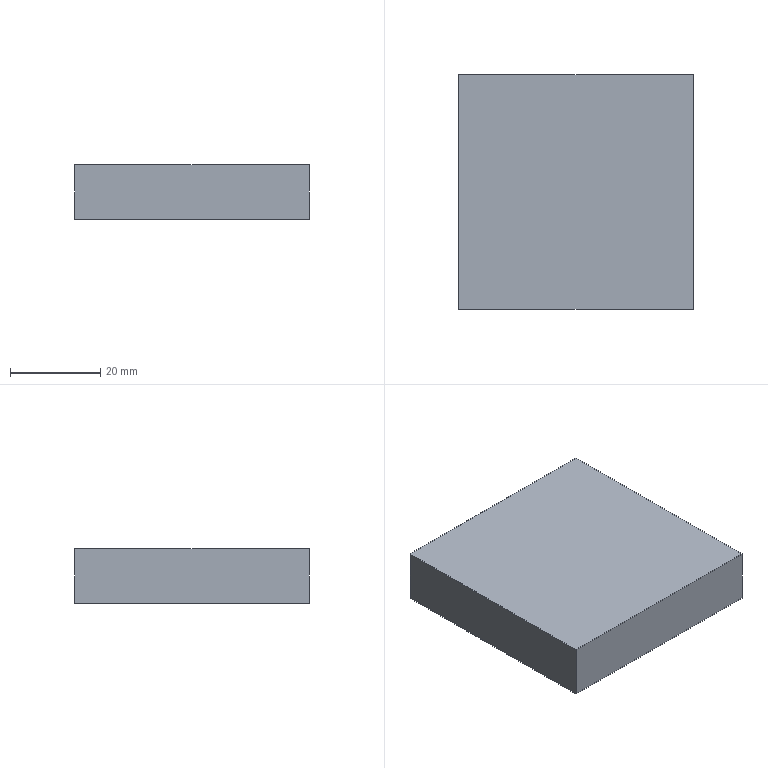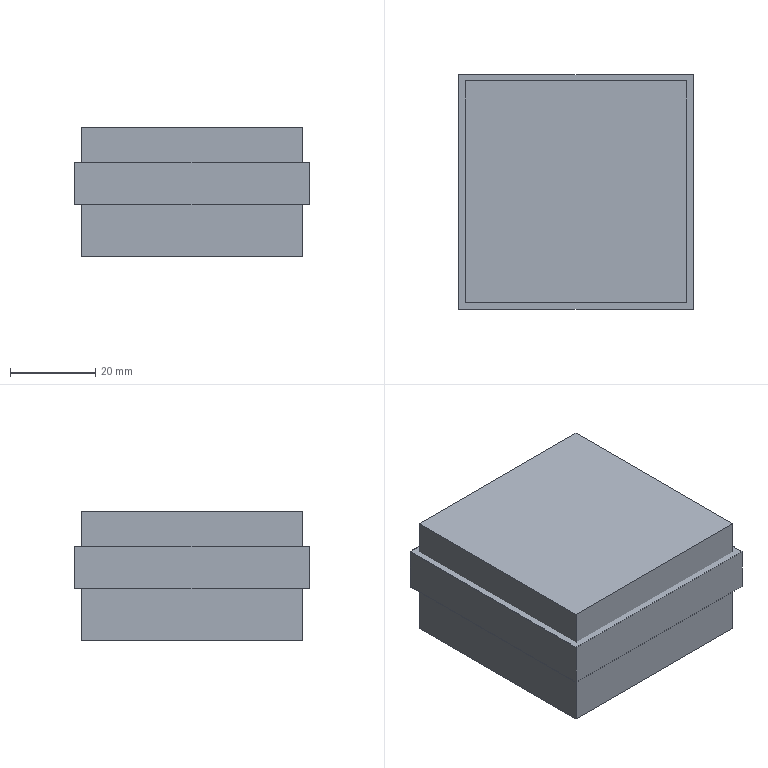CAM job | NX | 3-axis milling, drilling | part box 52 x 52 x 12 mm | stock box 55 x 55 x 30 mm
Tools:
number,name,description,diameter,corner_radius,flute_length,length,flutes
2,D4-12-D4-50-3T--FINISH,D4-12-D4-50-3T,4.0,0.0,12.0,50.0,3
1,D50面刀,D50面刀,50.0,0.0,30.0,30.0,4
4,钻头D3.3-45-73,钻刀D3.3-45-73,3.3,0.0,45.0,73.0,2
0,倒角D3-90度,倒角D3-90度,3.0,0.0,5.0,50.0,2
3,倒角D10-90度,倒角D10-90度,10.0,0.0,10.0,75.0,2
Operations:
program,operation,operation_type,tool,method,geometry_group,spindle_rpm,surface_speed,feed_per_tooth,feed_cut,feed_plunge,cut_length_mm,path_length_mm,cut_time_min,machine_time_min
A1,PLANAR_MILL,PlanarMilling,D50面刀,METHOD,A-G54,4500.0,706.0,0.0444,800.0,100.0,115.0,169.0,0.1437,0.1492
A1,ADAPTIVE_MILLING,CavityMilling,D4-12-D4-50-3T--FINISH,METHOD,WORKPIECE_54,6500.0,163.0,0.1923,2500.0,100.0,8077.867,8227.408,2.778,2.793
A1,PLANAR_MILL_1,PlanarMilling,D4-12-D4-50-3T--FINISH,METHOD,WORKPIECE_54,7500.0,94.0,0.0356,800.0,100.0,333.297,403.297,0.4166,0.4236
A1,PLANAR_MILL_1_COPY_1,PlanarMilling,D4-12-D4-50-3T--FINISH,METHOD,WORKPIECE_54,7500.0,94.0,0.0356,800.0,100.0,162.376,232.376,0.203,0.21
A1,PLANAR_MILL_1_COPY,PlanarMilling,倒角D3-90度,METHOD,WORKPIECE_54,3000.0,94.0,0.1333,800.0,100.0,156.905,214.905,0.1961,0.2019
A1,PLANAR_MILL_1_COPY_COPY,PlanarMilling,倒角D3-90度,METHOD,WORKPIECE_54,3000.0,94.0,0.1333,800.0,100.0,90.769,148.769,0.1135,0.1193
A1,DRILLING,Operation,倒角D10-90度,METHOD,WORKPIECE_54,1600.0,50.0,0.0625,200.0,0.0,28.6,143.99,0.143,0.1545
A1,DRILLING_COPY,Operation,钻头D3.3-45-73,METHOD,WORKPIECE_54,1600.0,16.0,0.0781,250.0,0.0,36.0,158.79,0.144,0.1563
A1,PLANAR_MILL_COPY,PlanarMilling,D50面刀,METHOD,A-G54,4500.0,706.0,0.0444,800.0,100.0,115.0,169.0,0.1437,0.1492
B1,ADAPTIVE_MILLING_2,CavityMilling,D4-12-D4-50-3T--FINISH,METHOD,WORKPIECE_55,6500.0,81.0,0.1282,2500.0,100.0,7601.422,7667.222,3.041,3.047
B1,PLANAR_MILL_4,PlanarMilling,倒角D3-90度,METHOD,WORKPIECE_55,4500.0,42.0,0.0889,800.0,100.0,90.769,148.769,0.1135,0.1193
B1,PLANAR_MILL_4_COPY,PlanarMilling,倒角D3-90度,METHOD,WORKPIECE_55,4500.0,42.0,0.0889,800.0,100.0,156.905,214.905,0.1961,0.2019
B1,PLANAR_MILL_3,PlanarMilling,D50面刀,METHOD,WORKPIECE_55,4500.0,706.0,0.0444,800.0,100.0,161.0,227.0,0.2012,0.2078
工装1,ADAPTIVE_MILLING_1,CavityMilling,D4-12-D4-50-3T--FINISH,METHOD,WORKPIECE,6500.0,81.0,0.1282,2500.0,100.0,4593.289,4629.589,1.497,1.501
工装1,FLOOR_FACING,VolumeBased25DMillingOperation,D4-12-D4-50-3T--FINISH,METHOD,WORKPIECE,4500.0,56.0,0.0593,800.0,100.0,430.594,474.594,0.5382,0.5426
工装1,PLANAR_MILL_2,PlanarMilling,D4-12-D4-50-3T--FINISH,METHOD,WORKPIECE,4500.0,56.0,0.0593,800.0,100.0,141.527,181.827,0.1769,0.1809